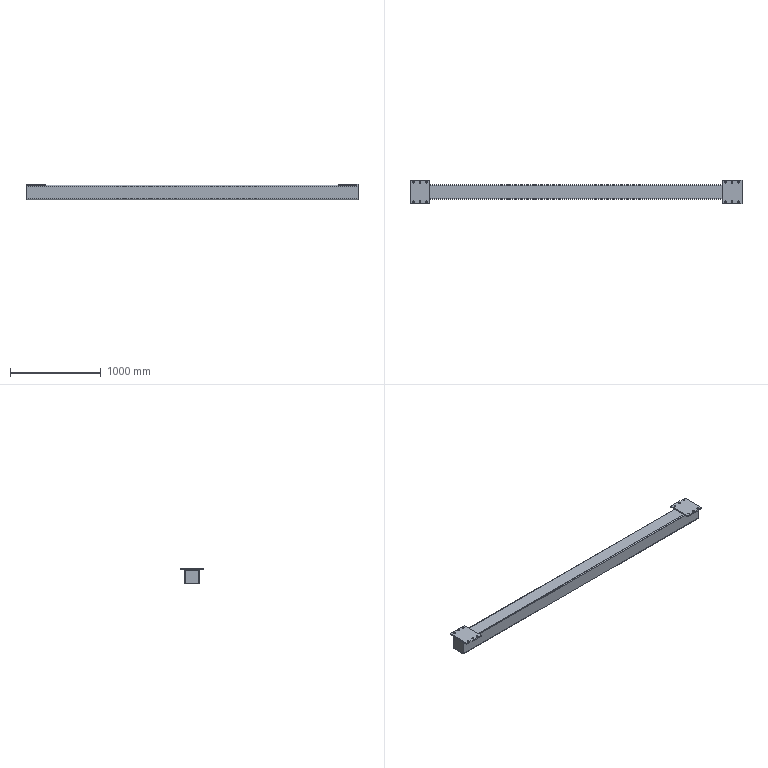Part | SolidWorks | features EndCap 2, HoleWzd 1, ICE 1, MirrorSolid 1, WeldMemberFeat 1, WeldmentFeature 1 | 5 solids | 66 faces | box 3659 x 260 x 174 mm | volume 12792331 mm3 | plane 34 | cylinder 32 | commonest cylinder face diameters 18 x24 10 x4 20 x4